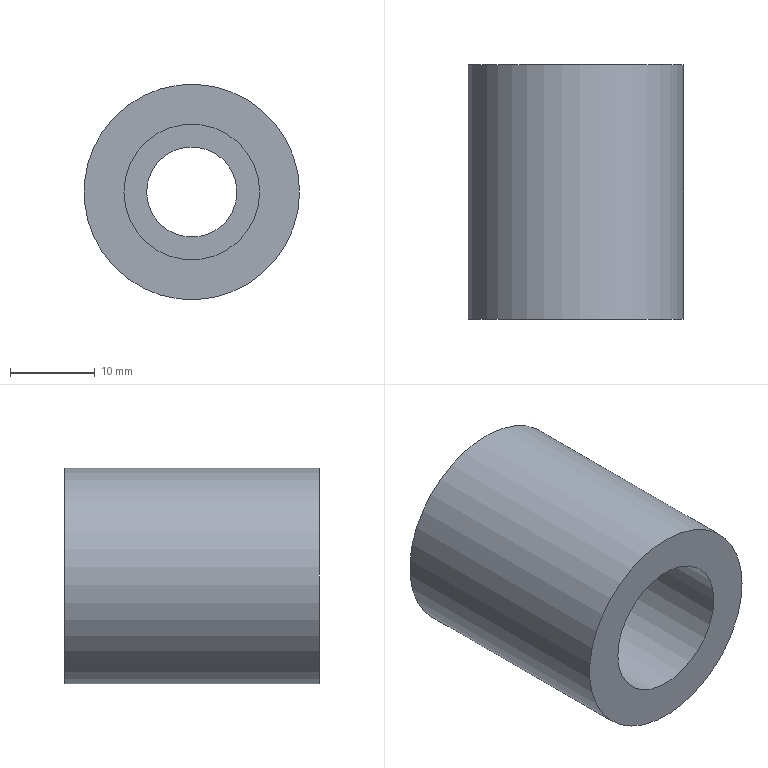Part | STEP file | 2_ESTAGIO_006-02 | 1 solid | 6 faces | box 25.4 x 30 x 25.4 mm | volume 10290 mm3 | plane 3 | cylinder 3 | commonest cylinder face diameters 10.647 x1 16 x1 25.4 x1
STEP:
#1=CARTESIAN_POINT('',(0.,0.,0.));
#2=DIRECTION('',(0.,0.,1.));
#3=DIRECTION('',(1.,0.,0.));
#4=AXIS2_PLACEMENT_3D('',#1,#2,#3);
#5=CARTESIAN_POINT('',(380.339,-512.65,377.849));
#6=VERTEX_POINT('',#5);
#7=CARTESIAN_POINT('',(388.339,-512.65,377.849));
#8=DIRECTION('',(0.,-1.,0.));
#9=DIRECTION('',(1.,0.,0.));
#10=AXIS2_PLACEMENT_3D('',#7,#8,#9);
#11=CIRCLE('',#10,8.);
#12=CARTESIAN_POINT('',(388.339,-512.65,377.849));
#13=DIRECTION('',(0.,-1.,0.));
#14=DIRECTION('',(0.,0.,-1.));
#15=AXIS2_PLACEMENT_3D('',#12,#13,#14);
#16=PLANE('',#15);
#17=CARTESIAN_POINT('',(0.,0.));
#18=DIRECTION('',(0.,1.));
#19=AXIS2_PLACEMENT_2D('',#17,#18);
#20=CIRCLE('',#19,8.);
#21=(GEOMETRIC_REPRESENTATION_CONTEXT(2)PARAMETRIC_REPRESENTATION_CONTEXT()REPRESENTATION_CONTEXT('',''));
#22=DEFINITIONAL_REPRESENTATION('',(#20),#21);
#23=PCURVE('',#16,#22);
#24=CARTESIAN_POINT('',(388.339,-523.31,377.849));
#25=DIRECTION('',(0.,1.,0.));
#26=DIRECTION('',(-1.,0.,0.));
#27=AXIS2_PLACEMENT_3D('',#24,#25,#26);
#28=CYLINDRICAL_SURFACE('',#27,8.);
#29=CARTESIAN_POINT('',(9.425,10.66));
#30=DIRECTION('',(-1.,0.));
#31=VECTOR('',#30,1.);
#32=LINE('',#29,#31);
#33=(GEOMETRIC_REPRESENTATION_CONTEXT(2)PARAMETRIC_REPRESENTATION_CONTEXT()REPRESENTATION_CONTEXT('',''));
#34=DEFINITIONAL_REPRESENTATION('',(#32),#33);
#35=PCURVE('',#28,#34);
#36=SURFACE_CURVE('',#11,(#23,#35),.PCURVE_S1.);
#37=EDGE_CURVE('',#6,#6,#36,.T.);
#38=ORIENTED_EDGE('',*,*,#37,.T.);
#39=EDGE_LOOP('',(#38));
#40=FACE_BOUND('',#39,.T.);
#41=CARTESIAN_POINT('',(393.011,-512.65,380.401));
#42=VERTEX_POINT('',#41);
#43=CARTESIAN_POINT('',(388.339,-512.65,377.849));
#44=DIRECTION('',(0.,-1.,0.));
#45=DIRECTION('',(1.,0.,0.));
#46=AXIS2_PLACEMENT_3D('',#43,#44,#45);
#47=CIRCLE('',#46,5.324);
#48=CARTESIAN_POINT('',(0.,0.));
#49=DIRECTION('',(0.,1.));
#50=AXIS2_PLACEMENT_2D('',#48,#49);
#51=CIRCLE('',#50,5.324);
#52=(GEOMETRIC_REPRESENTATION_CONTEXT(2)PARAMETRIC_REPRESENTATION_CONTEXT()REPRESENTATION_CONTEXT('',''));
#53=DEFINITIONAL_REPRESENTATION('',(#51),#52);
#54=PCURVE('',#16,#53);
#55=CARTESIAN_POINT('',(388.339,-502.75,377.849));
#56=DIRECTION('',(0.,-1.,0.));
#57=DIRECTION('',(0.8776,0.,0.4794));
#58=AXIS2_PLACEMENT_3D('',#55,#56,#57);
#59=CYLINDRICAL_SURFACE('',#58,5.324);
#60=CARTESIAN_POINT('',(-0.5,9.9));
#61=DIRECTION('',(1.,0.));
#62=VECTOR('',#61,1.);
#63=LINE('',#60,#62);
#64=(GEOMETRIC_REPRESENTATION_CONTEXT(2)PARAMETRIC_REPRESENTATION_CONTEXT()REPRESENTATION_CONTEXT('',''));
#65=DEFINITIONAL_REPRESENTATION('',(#63),#64);
#66=PCURVE('',#59,#65);
#67=SURFACE_CURVE('',#47,(#54,#66),.PCURVE_S1.);
#68=EDGE_CURVE('',#42,#42,#67,.T.);
#69=ORIENTED_EDGE('',*,*,#68,.F.);
#70=EDGE_LOOP('',(#69));
#71=FACE_BOUND('',#70,.T.);
#72=ADVANCED_FACE('',(#40,#71),#16,.T.);
#73=CARTESIAN_POINT('',(401.039,-502.65,377.849));
#74=VERTEX_POINT('',#73);
#75=CARTESIAN_POINT('',(388.339,-502.65,377.849));
#76=DIRECTION('',(0.,1.,0.));
#77=DIRECTION('',(1.,0.,0.));
#78=AXIS2_PLACEMENT_3D('',#75,#76,#77);
#79=CIRCLE('',#78,12.7);
#80=CARTESIAN_POINT('',(0.,-502.65,0.));
#81=DIRECTION('',(0.,1.,0.));
#82=DIRECTION('',(0.,0.,1.));
#83=AXIS2_PLACEMENT_3D('',#80,#81,#82);
#84=PLANE('',#83);
#85=CARTESIAN_POINT('',(377.849,388.339));
#86=DIRECTION('',(0.,1.));
#87=AXIS2_PLACEMENT_2D('',#85,#86);
#88=CIRCLE('',#87,12.7);
#89=(GEOMETRIC_REPRESENTATION_CONTEXT(2)PARAMETRIC_REPRESENTATION_CONTEXT()REPRESENTATION_CONTEXT('',''));
#90=DEFINITIONAL_REPRESENTATION('',(#88),#89);
#91=PCURVE('',#84,#90);
#92=CARTESIAN_POINT('',(388.339,-517.65,377.849));
#93=DIRECTION('',(0.,1.,0.));
#94=DIRECTION('',(-1.,0.,0.));
#95=AXIS2_PLACEMENT_3D('',#92,#93,#94);
#96=CYLINDRICAL_SURFACE('',#95,12.7);
#97=CARTESIAN_POINT('',(3.142,15.));
#98=DIRECTION('',(1.,0.));
#99=VECTOR('',#98,1.);
#100=LINE('',#97,#99);
#101=(GEOMETRIC_REPRESENTATION_CONTEXT(2)PARAMETRIC_REPRESENTATION_CONTEXT()REPRESENTATION_CONTEXT('',''));
#102=DEFINITIONAL_REPRESENTATION('',(#100),#101);
#103=PCURVE('',#96,#102);
#104=SURFACE_CURVE('',#79,(#91,#103),.PCURVE_S1.);
#105=EDGE_CURVE('',#74,#74,#104,.T.);
#106=ORIENTED_EDGE('',*,*,#105,.T.);
#107=EDGE_LOOP('',(#106));
#108=FACE_BOUND('',#107,.T.);
#109=CARTESIAN_POINT('',(393.011,-502.65,380.401));
#110=VERTEX_POINT('',#109);
#111=CARTESIAN_POINT('',(388.339,-502.65,377.849));
#112=DIRECTION('',(0.,1.,0.));
#113=DIRECTION('',(1.,0.,0.));
#114=AXIS2_PLACEMENT_3D('',#111,#112,#113);
#115=CIRCLE('',#114,5.324);
#116=CARTESIAN_POINT('',(377.849,388.339));
#117=DIRECTION('',(0.,1.));
#118=AXIS2_PLACEMENT_2D('',#116,#117);
#119=CIRCLE('',#118,5.324);
#120=(GEOMETRIC_REPRESENTATION_CONTEXT(2)PARAMETRIC_REPRESENTATION_CONTEXT()REPRESENTATION_CONTEXT('',''));
#121=DEFINITIONAL_REPRESENTATION('',(#119),#120);
#122=PCURVE('',#84,#121);
#123=CARTESIAN_POINT('',(12.066,-0.1));
#124=DIRECTION('',(-1.,0.));
#125=VECTOR('',#124,1.);
#126=LINE('',#123,#125);
#127=(GEOMETRIC_REPRESENTATION_CONTEXT(2)PARAMETRIC_REPRESENTATION_CONTEXT()REPRESENTATION_CONTEXT('',''));
#128=DEFINITIONAL_REPRESENTATION('',(#126),#127);
#129=PCURVE('',#59,#128);
#130=SURFACE_CURVE('',#115,(#122,#129),.PCURVE_S1.);
#131=EDGE_CURVE('',#110,#110,#130,.T.);
#132=ORIENTED_EDGE('',*,*,#131,.F.);
#133=EDGE_LOOP('',(#132));
#134=FACE_BOUND('',#133,.T.);
#135=ADVANCED_FACE('',(#108,#134),#84,.T.);
#136=ORIENTED_EDGE('',*,*,#105,.F.);
#137=CARTESIAN_POINT('',(401.039,-532.65,377.849));
#138=VERTEX_POINT('',#137);
#139=CARTESIAN_POINT('',(401.039,-532.65,377.849));
#140=CARTESIAN_POINT('',(401.039,-502.65,377.849));
#141=B_SPLINE_CURVE_WITH_KNOTS('',1,(#139,#140),.UNSPECIFIED.,.F.,.F.,(2,2),(-15.,15.),.PIECEWISE_BEZIER_KNOTS.);
#142=CARTESIAN_POINT('',(3.142,0.));
#143=DIRECTION('',(0.,1.));
#144=VECTOR('',#143,1.);
#145=LINE('',#142,#144);
#146=(GEOMETRIC_REPRESENTATION_CONTEXT(2)PARAMETRIC_REPRESENTATION_CONTEXT()REPRESENTATION_CONTEXT('',''));
#147=DEFINITIONAL_REPRESENTATION('',(#145),#146);
#148=PCURVE('',#96,#147);
#149=CARTESIAN_POINT('',(9.425,0.));
#150=DIRECTION('',(0.,1.));
#151=VECTOR('',#150,1.);
#152=LINE('',#149,#151);
#153=(GEOMETRIC_REPRESENTATION_CONTEXT(2)PARAMETRIC_REPRESENTATION_CONTEXT()REPRESENTATION_CONTEXT('',''));
#154=DEFINITIONAL_REPRESENTATION('',(#152),#153);
#155=PCURVE('',#96,#154);
#156=SEAM_CURVE('',#141,(#148,#155),.PCURVE_S1.);
#157=EDGE_CURVE('',#138,#74,#156,.T.);
#158=ORIENTED_EDGE('',*,*,#157,.F.);
#159=CARTESIAN_POINT('',(388.339,-532.65,377.849));
#160=DIRECTION('',(0.,1.,0.));
#161=DIRECTION('',(1.,0.,0.));
#162=AXIS2_PLACEMENT_3D('',#159,#160,#161);
#163=CIRCLE('',#162,12.7);
#164=CARTESIAN_POINT('',(3.142,-15.));
#165=DIRECTION('',(1.,0.));
#166=VECTOR('',#165,1.);
#167=LINE('',#164,#166);
#168=(GEOMETRIC_REPRESENTATION_CONTEXT(2)PARAMETRIC_REPRESENTATION_CONTEXT()REPRESENTATION_CONTEXT('',''));
#169=DEFINITIONAL_REPRESENTATION('',(#167),#168);
#170=PCURVE('',#96,#169);
#171=CARTESIAN_POINT('',(0.,-532.65,0.));
#172=DIRECTION('',(0.,1.,0.));
#173=DIRECTION('',(0.,0.,1.));
#174=AXIS2_PLACEMENT_3D('',#171,#172,#173);
#175=PLANE('',#174);
#176=CARTESIAN_POINT('',(377.849,388.339));
#177=DIRECTION('',(0.,1.));
#178=AXIS2_PLACEMENT_2D('',#176,#177);
#179=CIRCLE('',#178,12.7);
#180=(GEOMETRIC_REPRESENTATION_CONTEXT(2)PARAMETRIC_REPRESENTATION_CONTEXT()REPRESENTATION_CONTEXT('',''));
#181=DEFINITIONAL_REPRESENTATION('',(#179),#180);
#182=PCURVE('',#175,#181);
#183=SURFACE_CURVE('',#163,(#170,#182),.PCURVE_S1.);
#184=EDGE_CURVE('',#138,#138,#183,.T.);
#185=ORIENTED_EDGE('',*,*,#184,.T.);
#186=ORIENTED_EDGE('',*,*,#157,.T.);
#187=EDGE_LOOP('',(#136,#158,#185,#186));
#188=FACE_BOUND('',#187,.T.);
#189=ADVANCED_FACE('',(#188),#96,.T.);
#190=ORIENTED_EDGE('',*,*,#184,.F.);
#191=EDGE_LOOP('',(#190));
#192=FACE_BOUND('',#191,.T.);
#193=CARTESIAN_POINT('',(380.339,-532.65,377.849));
#194=VERTEX_POINT('',#193);
#195=CARTESIAN_POINT('',(388.339,-532.65,377.849));
#196=DIRECTION('',(0.,1.,0.));
#197=DIRECTION('',(1.,0.,0.));
#198=AXIS2_PLACEMENT_3D('',#195,#196,#197);
#199=CIRCLE('',#198,8.);
#200=CARTESIAN_POINT('',(377.849,388.339));
#201=DIRECTION('',(0.,1.));
#202=AXIS2_PLACEMENT_2D('',#200,#201);
#203=CIRCLE('',#202,8.);
#204=(GEOMETRIC_REPRESENTATION_CONTEXT(2)PARAMETRIC_REPRESENTATION_CONTEXT()REPRESENTATION_CONTEXT('',''));
#205=DEFINITIONAL_REPRESENTATION('',(#203),#204);
#206=PCURVE('',#175,#205);
#207=CARTESIAN_POINT('',(-3.142,-9.34));
#208=DIRECTION('',(1.,0.));
#209=VECTOR('',#208,1.);
#210=LINE('',#207,#209);
#211=(GEOMETRIC_REPRESENTATION_CONTEXT(2)PARAMETRIC_REPRESENTATION_CONTEXT()REPRESENTATION_CONTEXT('',''));
#212=DEFINITIONAL_REPRESENTATION('',(#210),#211);
#213=PCURVE('',#28,#212);
#214=SURFACE_CURVE('',#199,(#206,#213),.PCURVE_S1.);
#215=EDGE_CURVE('',#194,#194,#214,.T.);
#216=ORIENTED_EDGE('',*,*,#215,.T.);
#217=EDGE_LOOP('',(#216));
#218=FACE_BOUND('',#217,.T.);
#219=ADVANCED_FACE('',(#192,#218),#175,.F.);
#220=ORIENTED_EDGE('',*,*,#131,.F.);
#221=CARTESIAN_POINT('',(393.011,-502.65,380.401));
#222=CARTESIAN_POINT('',(393.011,-512.65,380.401));
#223=B_SPLINE_CURVE_WITH_KNOTS('',1,(#221,#222),.UNSPECIFIED.,.F.,.F.,(2,2),(-0.1,9.9),.PIECEWISE_BEZIER_KNOTS.);
#224=CARTESIAN_POINT('',(6.283,0.));
#225=DIRECTION('',(0.,1.));
#226=VECTOR('',#225,1.);
#227=LINE('',#224,#226);
#228=(GEOMETRIC_REPRESENTATION_CONTEXT(2)PARAMETRIC_REPRESENTATION_CONTEXT()REPRESENTATION_CONTEXT('',''));
#229=DEFINITIONAL_REPRESENTATION('',(#227),#228);
#230=PCURVE('',#59,#229);
#231=CARTESIAN_POINT('',(0.,0.));
#232=DIRECTION('',(0.,1.));
#233=VECTOR('',#232,1.);
#234=LINE('',#231,#233);
#235=(GEOMETRIC_REPRESENTATION_CONTEXT(2)PARAMETRIC_REPRESENTATION_CONTEXT()REPRESENTATION_CONTEXT('',''));
#236=DEFINITIONAL_REPRESENTATION('',(#234),#235);
#237=PCURVE('',#59,#236);
#238=SEAM_CURVE('',#223,(#230,#237),.PCURVE_S1.);
#239=EDGE_CURVE('',#110,#42,#238,.T.);
#240=ORIENTED_EDGE('',*,*,#239,.T.);
#241=ORIENTED_EDGE('',*,*,#68,.F.);
#242=ORIENTED_EDGE('',*,*,#239,.F.);
#243=EDGE_LOOP('',(#220,#240,#241,#242));
#244=FACE_BOUND('',#243,.F.);
#245=ADVANCED_FACE('',(#244),#59,.F.);
#246=ORIENTED_EDGE('',*,*,#215,.T.);
#247=CARTESIAN_POINT('',(380.339,-532.65,377.849));
#248=CARTESIAN_POINT('',(380.339,-512.65,377.849));
#249=B_SPLINE_CURVE_WITH_KNOTS('',1,(#247,#248),.UNSPECIFIED.,.F.,.F.,(2,2),(-9.34,10.66),.PIECEWISE_BEZIER_KNOTS.);
#250=CARTESIAN_POINT('',(6.283,0.));
#251=DIRECTION('',(0.,1.));
#252=VECTOR('',#251,1.);
#253=LINE('',#250,#252);
#254=(GEOMETRIC_REPRESENTATION_CONTEXT(2)PARAMETRIC_REPRESENTATION_CONTEXT()REPRESENTATION_CONTEXT('',''));
#255=DEFINITIONAL_REPRESENTATION('',(#253),#254);
#256=PCURVE('',#28,#255);
#257=CARTESIAN_POINT('',(0.,0.));
#258=DIRECTION('',(0.,1.));
#259=VECTOR('',#258,1.);
#260=LINE('',#257,#259);
#261=(GEOMETRIC_REPRESENTATION_CONTEXT(2)PARAMETRIC_REPRESENTATION_CONTEXT()REPRESENTATION_CONTEXT('',''));
#262=DEFINITIONAL_REPRESENTATION('',(#260),#261);
#263=PCURVE('',#28,#262);
#264=SEAM_CURVE('',#249,(#256,#263),.PCURVE_S1.);
#265=EDGE_CURVE('',#194,#6,#264,.T.);
#266=ORIENTED_EDGE('',*,*,#265,.T.);
#267=ORIENTED_EDGE('',*,*,#37,.T.);
#268=ORIENTED_EDGE('',*,*,#265,.F.);
#269=EDGE_LOOP('',(#246,#266,#267,#268));
#270=FACE_BOUND('',#269,.F.);
#271=ADVANCED_FACE('',(#270),#28,.F.);
#272=CLOSED_SHELL('',(#72,#135,#189,#219,#245,#271));
#273=MANIFOLD_SOLID_BREP('',#272);
#274=(LENGTH_UNIT()NAMED_UNIT(*)SI_UNIT(.MILLI.,.METRE.));
#275=UNCERTAINTY_MEASURE_WITH_UNIT(LENGTH_MEASURE(0.00001),#274,'','');
#276=(NAMED_UNIT(*)PLANE_ANGLE_UNIT()SI_UNIT($,.RADIAN.));
#277=(NAMED_UNIT(*)SI_UNIT($,.STERADIAN.)SOLID_ANGLE_UNIT());
#278=(GEOMETRIC_REPRESENTATION_CONTEXT(3)GLOBAL_UNCERTAINTY_ASSIGNED_CONTEXT((#275))GLOBAL_UNIT_ASSIGNED_CONTEXT((#274,#276,#277))REPRESENTATION_CONTEXT('',''));
#279=ADVANCED_BREP_SHAPE_REPRESENTATION('',(#4,#273),#278);